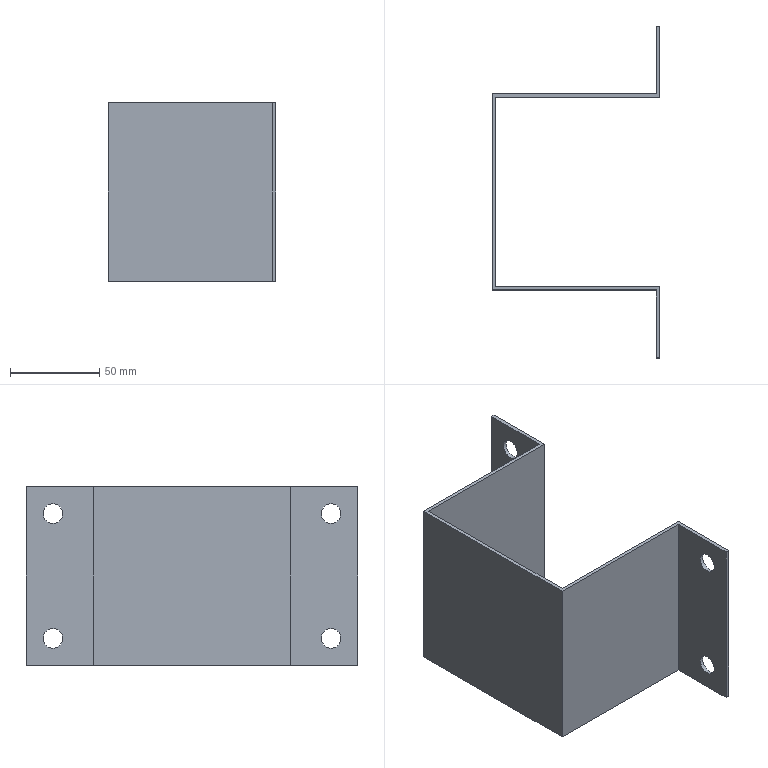Part | NX | features solid 2 | 1 solid | 18 faces | box 94 x 186 x 100 mm | volume 73240 mm3 | plane 14 | cylinder 4 | commonest cylinder face diameters 11 x4
STEP:
#1=CARTESIAN_POINT('',(1132.,-77.,-389.5));
#2=VERTEX_POINT('',#1);
#3=CARTESIAN_POINT('',(1132.,-77.,-395.));
#4=DIRECTION('',(-1.,0.,0.));
#5=DIRECTION('',(0.,0.,1.));
#6=AXIS2_PLACEMENT_3D('',#3,#4,#5);
#7=CIRCLE('',#6,5.5);
#8=EDGE_CURVE('',#2,#2,#7,.F.);
#9=ORIENTED_EDGE('',*,*,#8,.F.);
#10=EDGE_LOOP('',(#9));
#11=FACE_BOUND('',#10,.T.);
#12=CARTESIAN_POINT('',(1132.,-102.,-480.));
#13=VERTEX_POINT('',#12);
#14=CARTESIAN_POINT('',(1132.,-62.,-480.));
#15=VERTEX_POINT('',#14);
#16=CARTESIAN_POINT('',(1132.,-74.,-480.));
#17=DIRECTION('',(0.,1.,0.));
#18=VECTOR('',#17,1000.);
#19=LINE('',#16,#18);
#20=EDGE_CURVE('',#13,#15,#19,.T.);
#21=ORIENTED_EDGE('',*,*,#20,.T.);
#22=CARTESIAN_POINT('',(1132.,-62.,-380.));
#23=VERTEX_POINT('',#22);
#24=CARTESIAN_POINT('',(1132.,-62.,-480.));
#25=DIRECTION('',(0.,0.,1.));
#26=VECTOR('',#25,1000.);
#27=LINE('',#24,#26);
#28=EDGE_CURVE('',#15,#23,#27,.T.);
#29=ORIENTED_EDGE('',*,*,#28,.T.);
#30=CARTESIAN_POINT('',(1132.,-102.,-380.));
#31=VERTEX_POINT('',#30);
#32=CARTESIAN_POINT('',(1132.,-74.,-380.));
#33=DIRECTION('',(0.,1.,0.));
#34=VECTOR('',#33,1000.);
#35=LINE('',#32,#34);
#36=EDGE_CURVE('',#31,#23,#35,.T.);
#37=ORIENTED_EDGE('',*,*,#36,.F.);
#38=CARTESIAN_POINT('',(1132.,-102.,-480.));
#39=DIRECTION('',(0.,0.,1.));
#40=VECTOR('',#39,1000.);
#41=LINE('',#38,#40);
#42=EDGE_CURVE('',#13,#31,#41,.T.);
#43=ORIENTED_EDGE('',*,*,#42,.F.);
#44=EDGE_LOOP('',(#21,#29,#37,#43));
#45=FACE_BOUND('',#44,.T.);
#46=CARTESIAN_POINT('',(1132.,-77.,-459.5));
#47=VERTEX_POINT('',#46);
#48=CARTESIAN_POINT('',(1132.,-77.,-465.));
#49=DIRECTION('',(-1.,0.,0.));
#50=DIRECTION('',(0.,0.,1.));
#51=AXIS2_PLACEMENT_3D('',#48,#49,#50);
#52=CIRCLE('',#51,5.5);
#53=EDGE_CURVE('',#47,#47,#52,.F.);
#54=ORIENTED_EDGE('',*,*,#53,.F.);
#55=EDGE_LOOP('',(#54));
#56=FACE_BOUND('',#55,.T.);
#57=CARTESIAN_POINT('',(1132.,-74.,-480.));
#58=DIRECTION('',(-1.,0.,0.));
#59=DIRECTION('',(0.,1.,0.));
#60=AXIS2_PLACEMENT_3D('',#57,#58,#59);
#61=PLANE('',#60);
#62=ADVANCED_FACE('',(#11,#45,#56),#61,.F.);
#63=CARTESIAN_POINT('',(1130.,-77.,-389.5));
#64=VERTEX_POINT('',#63);
#65=CARTESIAN_POINT('',(1130.,-77.,-395.));
#66=DIRECTION('',(-1.,0.,0.));
#67=DIRECTION('',(0.,0.,1.));
#68=AXIS2_PLACEMENT_3D('',#65,#66,#67);
#69=CIRCLE('',#68,5.5);
#70=EDGE_CURVE('',#64,#64,#69,.F.);
#71=ORIENTED_EDGE('',*,*,#70,.T.);
#72=EDGE_LOOP('',(#71));
#73=FACE_BOUND('',#72,.T.);
#74=CARTESIAN_POINT('',(1130.,-100.,-480.));
#75=VERTEX_POINT('',#74);
#76=CARTESIAN_POINT('',(1130.,-62.,-480.));
#77=VERTEX_POINT('',#76);
#78=CARTESIAN_POINT('',(1130.,-72.,-480.));
#79=DIRECTION('',(0.,1.,0.));
#80=VECTOR('',#79,1000.);
#81=LINE('',#78,#80);
#82=EDGE_CURVE('',#75,#77,#81,.T.);
#83=ORIENTED_EDGE('',*,*,#82,.F.);
#84=CARTESIAN_POINT('',(1130.,-100.,-380.));
#85=VERTEX_POINT('',#84);
#86=CARTESIAN_POINT('',(1130.,-100.,-480.));
#87=DIRECTION('',(0.,0.,1.));
#88=VECTOR('',#87,1000.);
#89=LINE('',#86,#88);
#90=EDGE_CURVE('',#75,#85,#89,.T.);
#91=ORIENTED_EDGE('',*,*,#90,.T.);
#92=CARTESIAN_POINT('',(1130.,-62.,-380.));
#93=VERTEX_POINT('',#92);
#94=CARTESIAN_POINT('',(1130.,-72.,-380.));
#95=DIRECTION('',(0.,1.,0.));
#96=VECTOR('',#95,1000.);
#97=LINE('',#94,#96);
#98=EDGE_CURVE('',#85,#93,#97,.T.);
#99=ORIENTED_EDGE('',*,*,#98,.T.);
#100=CARTESIAN_POINT('',(1130.,-62.,-480.));
#101=DIRECTION('',(0.,0.,1.));
#102=VECTOR('',#101,1000.);
#103=LINE('',#100,#102);
#104=EDGE_CURVE('',#77,#93,#103,.T.);
#105=ORIENTED_EDGE('',*,*,#104,.F.);
#106=EDGE_LOOP('',(#83,#91,#99,#105));
#107=FACE_BOUND('',#106,.T.);
#108=CARTESIAN_POINT('',(1130.,-77.,-459.5));
#109=VERTEX_POINT('',#108);
#110=CARTESIAN_POINT('',(1130.,-77.,-465.));
#111=DIRECTION('',(-1.,0.,0.));
#112=DIRECTION('',(0.,0.,1.));
#113=AXIS2_PLACEMENT_3D('',#110,#111,#112);
#114=CIRCLE('',#113,5.5);
#115=EDGE_CURVE('',#109,#109,#114,.F.);
#116=ORIENTED_EDGE('',*,*,#115,.T.);
#117=EDGE_LOOP('',(#116));
#118=FACE_BOUND('',#117,.T.);
#119=CARTESIAN_POINT('',(1130.,-72.,-480.));
#120=DIRECTION('',(-1.,0.,0.));
#121=DIRECTION('',(0.,0.,1.));
#122=AXIS2_PLACEMENT_3D('',#119,#120,#121);
#123=PLANE('',#122);
#124=ADVANCED_FACE('',(#73,#107,#118),#123,.T.);
#125=CARTESIAN_POINT('',(1132.,-233.,-389.5));
#126=VERTEX_POINT('',#125);
#127=CARTESIAN_POINT('',(1132.,-233.,-395.));
#128=DIRECTION('',(-1.,0.,0.));
#129=DIRECTION('',(0.,0.,1.));
#130=AXIS2_PLACEMENT_3D('',#127,#128,#129);
#131=CIRCLE('',#130,5.5);
#132=EDGE_CURVE('',#126,#126,#131,.T.);
#133=ORIENTED_EDGE('',*,*,#132,.T.);
#134=EDGE_LOOP('',(#133));
#135=FACE_BOUND('',#134,.T.);
#136=CARTESIAN_POINT('',(1132.,-208.,-380.));
#137=VERTEX_POINT('',#136);
#138=CARTESIAN_POINT('',(1132.,-248.,-380.));
#139=VERTEX_POINT('',#138);
#140=CARTESIAN_POINT('',(1132.,-206.,-380.));
#141=DIRECTION('',(0.,1.,0.));
#142=VECTOR('',#141,1000.);
#143=LINE('',#140,#142);
#144=EDGE_CURVE('',#137,#139,#143,.F.);
#145=ORIENTED_EDGE('',*,*,#144,.T.);
#146=CARTESIAN_POINT('',(1132.,-248.,-480.));
#147=VERTEX_POINT('',#146);
#148=CARTESIAN_POINT('',(1132.,-248.,-480.));
#149=DIRECTION('',(0.,0.,1.));
#150=VECTOR('',#149,1000.);
#151=LINE('',#148,#150);
#152=EDGE_CURVE('',#147,#139,#151,.T.);
#153=ORIENTED_EDGE('',*,*,#152,.F.);
#154=CARTESIAN_POINT('',(1132.,-208.,-480.));
#155=VERTEX_POINT('',#154);
#156=CARTESIAN_POINT('',(1132.,-206.,-480.));
#157=DIRECTION('',(0.,1.,0.));
#158=VECTOR('',#157,1000.);
#159=LINE('',#156,#158);
#160=EDGE_CURVE('',#155,#147,#159,.F.);
#161=ORIENTED_EDGE('',*,*,#160,.F.);
#162=CARTESIAN_POINT('',(1132.,-208.,-480.));
#163=DIRECTION('',(0.,0.,-1.));
#164=VECTOR('',#163,1000.);
#165=LINE('',#162,#164);
#166=EDGE_CURVE('',#155,#137,#165,.F.);
#167=ORIENTED_EDGE('',*,*,#166,.T.);
#168=EDGE_LOOP('',(#145,#153,#161,#167));
#169=FACE_BOUND('',#168,.T.);
#170=CARTESIAN_POINT('',(1132.,-233.,-459.5));
#171=VERTEX_POINT('',#170);
#172=CARTESIAN_POINT('',(1132.,-233.,-465.));
#173=DIRECTION('',(-1.,0.,0.));
#174=DIRECTION('',(0.,0.,1.));
#175=AXIS2_PLACEMENT_3D('',#172,#173,#174);
#176=CIRCLE('',#175,5.5);
#177=EDGE_CURVE('',#171,#171,#176,.T.);
#178=ORIENTED_EDGE('',*,*,#177,.T.);
#179=EDGE_LOOP('',(#178));
#180=FACE_BOUND('',#179,.T.);
#181=CARTESIAN_POINT('',(1132.,-106.,-480.));
#182=DIRECTION('',(-1.,0.,0.));
#183=DIRECTION('',(0.,1.,0.));
#184=AXIS2_PLACEMENT_3D('',#181,#182,#183);
#185=PLANE('',#184);
#186=ADVANCED_FACE('',(#135,#169,#180),#185,.F.);
#187=CARTESIAN_POINT('',(1130.,-233.,-389.5));
#188=VERTEX_POINT('',#187);
#189=CARTESIAN_POINT('',(1130.,-233.,-395.));
#190=DIRECTION('',(-1.,0.,0.));
#191=DIRECTION('',(0.,0.,1.));
#192=AXIS2_PLACEMENT_3D('',#189,#190,#191);
#193=CIRCLE('',#192,5.5);
#194=EDGE_CURVE('',#188,#188,#193,.T.);
#195=ORIENTED_EDGE('',*,*,#194,.F.);
#196=EDGE_LOOP('',(#195));
#197=FACE_BOUND('',#196,.T.);
#198=CARTESIAN_POINT('',(1130.,-210.,-380.));
#199=VERTEX_POINT('',#198);
#200=CARTESIAN_POINT('',(1130.,-248.,-380.));
#201=VERTEX_POINT('',#200);
#202=CARTESIAN_POINT('',(1130.,-208.,-380.));
#203=DIRECTION('',(0.,1.,0.));
#204=VECTOR('',#203,1000.);
#205=LINE('',#202,#204);
#206=EDGE_CURVE('',#199,#201,#205,.F.);
#207=ORIENTED_EDGE('',*,*,#206,.F.);
#208=CARTESIAN_POINT('',(1130.,-210.,-480.));
#209=VERTEX_POINT('',#208);
#210=CARTESIAN_POINT('',(1130.,-210.,-480.));
#211=DIRECTION('',(0.,0.,1.));
#212=VECTOR('',#211,1000.);
#213=LINE('',#210,#212);
#214=EDGE_CURVE('',#199,#209,#213,.F.);
#215=ORIENTED_EDGE('',*,*,#214,.T.);
#216=CARTESIAN_POINT('',(1130.,-248.,-480.));
#217=VERTEX_POINT('',#216);
#218=CARTESIAN_POINT('',(1130.,-208.,-480.));
#219=DIRECTION('',(0.,1.,0.));
#220=VECTOR('',#219,1000.);
#221=LINE('',#218,#220);
#222=EDGE_CURVE('',#209,#217,#221,.F.);
#223=ORIENTED_EDGE('',*,*,#222,.T.);
#224=CARTESIAN_POINT('',(1130.,-248.,-480.));
#225=DIRECTION('',(0.,0.,-1.));
#226=VECTOR('',#225,1000.);
#227=LINE('',#224,#226);
#228=EDGE_CURVE('',#217,#201,#227,.F.);
#229=ORIENTED_EDGE('',*,*,#228,.T.);
#230=EDGE_LOOP('',(#207,#215,#223,#229));
#231=FACE_BOUND('',#230,.T.);
#232=CARTESIAN_POINT('',(1130.,-233.,-459.5));
#233=VERTEX_POINT('',#232);
#234=CARTESIAN_POINT('',(1130.,-233.,-465.));
#235=DIRECTION('',(-1.,0.,0.));
#236=DIRECTION('',(0.,0.,1.));
#237=AXIS2_PLACEMENT_3D('',#234,#235,#236);
#238=CIRCLE('',#237,5.5);
#239=EDGE_CURVE('',#233,#233,#238,.T.);
#240=ORIENTED_EDGE('',*,*,#239,.F.);
#241=EDGE_LOOP('',(#240));
#242=FACE_BOUND('',#241,.T.);
#243=CARTESIAN_POINT('',(1130.,-208.,-480.));
#244=DIRECTION('',(-1.,0.,0.));
#245=DIRECTION('',(0.,0.,1.));
#246=AXIS2_PLACEMENT_3D('',#243,#244,#245);
#247=PLANE('',#246);
#248=ADVANCED_FACE('',(#197,#231,#242),#247,.T.);
#249=CARTESIAN_POINT('',(1038.,-100.,-480.));
#250=VERTEX_POINT('',#249);
#251=CARTESIAN_POINT('',(1040.,-100.,-480.));
#252=DIRECTION('',(1.,0.,0.));
#253=VECTOR('',#252,1000.);
#254=LINE('',#251,#253);
#255=EDGE_CURVE('',#250,#75,#254,.T.);
#256=ORIENTED_EDGE('',*,*,#255,.T.);
#257=ORIENTED_EDGE('',*,*,#82,.T.);
#258=CARTESIAN_POINT('',(1130.,-62.,-480.));
#259=DIRECTION('',(1.,0.,0.));
#260=VECTOR('',#259,1000.);
#261=LINE('',#258,#260);
#262=EDGE_CURVE('',#77,#15,#261,.T.);
#263=ORIENTED_EDGE('',*,*,#262,.T.);
#264=ORIENTED_EDGE('',*,*,#20,.F.);
#265=CARTESIAN_POINT('',(1040.,-102.,-480.));
#266=VERTEX_POINT('',#265);
#267=CARTESIAN_POINT('',(1040.,-102.,-480.));
#268=DIRECTION('',(1.,0.,0.));
#269=VECTOR('',#268,1000.);
#270=LINE('',#267,#269);
#271=EDGE_CURVE('',#266,#13,#270,.T.);
#272=ORIENTED_EDGE('',*,*,#271,.F.);
#273=CARTESIAN_POINT('',(1040.,-208.,-480.));
#274=VERTEX_POINT('',#273);
#275=CARTESIAN_POINT('',(1040.,-206.,-480.));
#276=DIRECTION('',(0.,1.,0.));
#277=VECTOR('',#276,1000.);
#278=LINE('',#275,#277);
#279=EDGE_CURVE('',#274,#266,#278,.T.);
#280=ORIENTED_EDGE('',*,*,#279,.F.);
#281=CARTESIAN_POINT('',(1040.,-208.,-480.));
#282=DIRECTION('',(1.,0.,0.));
#283=VECTOR('',#282,1000.);
#284=LINE('',#281,#283);
#285=EDGE_CURVE('',#274,#155,#284,.T.);
#286=ORIENTED_EDGE('',*,*,#285,.T.);
#287=ORIENTED_EDGE('',*,*,#160,.T.);
#288=CARTESIAN_POINT('',(1130.,-248.,-480.));
#289=DIRECTION('',(1.,0.,0.));
#290=VECTOR('',#289,1000.);
#291=LINE('',#288,#290);
#292=EDGE_CURVE('',#217,#147,#291,.T.);
#293=ORIENTED_EDGE('',*,*,#292,.F.);
#294=ORIENTED_EDGE('',*,*,#222,.F.);
#295=CARTESIAN_POINT('',(1038.,-210.,-480.));
#296=VERTEX_POINT('',#295);
#297=CARTESIAN_POINT('',(1040.,-210.,-480.));
#298=DIRECTION('',(-1.,0.,0.));
#299=VECTOR('',#298,1000.);
#300=LINE('',#297,#299);
#301=EDGE_CURVE('',#296,#209,#300,.F.);
#302=ORIENTED_EDGE('',*,*,#301,.F.);
#303=CARTESIAN_POINT('',(1038.,-206.,-480.));
#304=DIRECTION('',(0.,-1.,0.));
#305=VECTOR('',#304,1000.);
#306=LINE('',#303,#305);
#307=EDGE_CURVE('',#296,#250,#306,.F.);
#308=ORIENTED_EDGE('',*,*,#307,.T.);
#309=EDGE_LOOP('',(#256,#257,#263,#264,#272,#280,#286,#287,#293,#294,#302,#308));
#310=FACE_BOUND('',#309,.T.);
#311=CARTESIAN_POINT('',(1040.,-74.,-480.));
#312=DIRECTION('',(0.,0.,1.));
#313=DIRECTION('',(-1.,0.,0.));
#314=AXIS2_PLACEMENT_3D('',#311,#312,#313);
#315=PLANE('',#314);
#316=ADVANCED_FACE('',(#310),#315,.F.);
#317=CARTESIAN_POINT('',(1040.,-102.,-380.));
#318=VERTEX_POINT('',#317);
#319=CARTESIAN_POINT('',(1040.,-102.,-380.));
#320=DIRECTION('',(1.,0.,0.));
#321=VECTOR('',#320,1000.);
#322=LINE('',#319,#321);
#323=EDGE_CURVE('',#318,#31,#322,.T.);
#324=ORIENTED_EDGE('',*,*,#323,.T.);
#325=ORIENTED_EDGE('',*,*,#36,.T.);
#326=CARTESIAN_POINT('',(1130.,-62.,-380.));
#327=DIRECTION('',(1.,0.,0.));
#328=VECTOR('',#327,1000.);
#329=LINE('',#326,#328);
#330=EDGE_CURVE('',#93,#23,#329,.T.);
#331=ORIENTED_EDGE('',*,*,#330,.F.);
#332=ORIENTED_EDGE('',*,*,#98,.F.);
#333=CARTESIAN_POINT('',(1038.,-100.,-380.));
#334=VERTEX_POINT('',#333);
#335=CARTESIAN_POINT('',(1040.,-100.,-380.));
#336=DIRECTION('',(1.,0.,0.));
#337=VECTOR('',#336,1000.);
#338=LINE('',#335,#337);
#339=EDGE_CURVE('',#334,#85,#338,.T.);
#340=ORIENTED_EDGE('',*,*,#339,.F.);
#341=CARTESIAN_POINT('',(1038.,-210.,-380.));
#342=VERTEX_POINT('',#341);
#343=CARTESIAN_POINT('',(1038.,-206.,-380.));
#344=DIRECTION('',(0.,1.,0.));
#345=VECTOR('',#344,1000.);
#346=LINE('',#343,#345);
#347=EDGE_CURVE('',#342,#334,#346,.T.);
#348=ORIENTED_EDGE('',*,*,#347,.F.);
#349=CARTESIAN_POINT('',(1040.,-210.,-380.));
#350=DIRECTION('',(1.,0.,0.));
#351=VECTOR('',#350,1000.);
#352=LINE('',#349,#351);
#353=EDGE_CURVE('',#342,#199,#352,.T.);
#354=ORIENTED_EDGE('',*,*,#353,.T.);
#355=ORIENTED_EDGE('',*,*,#206,.T.);
#356=CARTESIAN_POINT('',(1130.,-248.,-380.));
#357=DIRECTION('',(-1.,0.,0.));
#358=VECTOR('',#357,1000.);
#359=LINE('',#356,#358);
#360=EDGE_CURVE('',#201,#139,#359,.F.);
#361=ORIENTED_EDGE('',*,*,#360,.T.);
#362=ORIENTED_EDGE('',*,*,#144,.F.);
#363=CARTESIAN_POINT('',(1040.,-208.,-380.));
#364=VERTEX_POINT('',#363);
#365=CARTESIAN_POINT('',(1040.,-208.,-380.));
#366=DIRECTION('',(1.,0.,0.));
#367=VECTOR('',#366,1000.);
#368=LINE('',#365,#367);
#369=EDGE_CURVE('',#364,#137,#368,.T.);
#370=ORIENTED_EDGE('',*,*,#369,.F.);
#371=CARTESIAN_POINT('',(1040.,-206.,-380.));
#372=DIRECTION('',(0.,-1.,0.));
#373=VECTOR('',#372,1000.);
#374=LINE('',#371,#373);
#375=EDGE_CURVE('',#364,#318,#374,.F.);
#376=ORIENTED_EDGE('',*,*,#375,.T.);
#377=EDGE_LOOP('',(#324,#325,#331,#332,#340,#348,#354,#355,#361,#362,#370,#376));
#378=FACE_BOUND('',#377,.T.);
#379=CARTESIAN_POINT('',(1040.,-74.,-380.));
#380=DIRECTION('',(0.,0.,1.));
#381=DIRECTION('',(-1.,0.,0.));
#382=AXIS2_PLACEMENT_3D('',#379,#380,#381);
#383=PLANE('',#382);
#384=ADVANCED_FACE('',(#378),#383,.T.);
#385=ORIENTED_EDGE('',*,*,#271,.T.);
#386=ORIENTED_EDGE('',*,*,#42,.T.);
#387=ORIENTED_EDGE('',*,*,#323,.F.);
#388=CARTESIAN_POINT('',(1040.,-102.,-480.));
#389=DIRECTION('',(0.,0.,1.));
#390=VECTOR('',#389,1000.);
#391=LINE('',#388,#390);
#392=EDGE_CURVE('',#266,#318,#391,.T.);
#393=ORIENTED_EDGE('',*,*,#392,.F.);
#394=EDGE_LOOP('',(#385,#386,#387,#393));
#395=FACE_BOUND('',#394,.T.);
#396=CARTESIAN_POINT('',(1040.,-102.,-480.));
#397=DIRECTION('',(0.,1.,0.));
#398=DIRECTION('',(1.,0.,0.));
#399=AXIS2_PLACEMENT_3D('',#396,#397,#398);
#400=PLANE('',#399);
#401=ADVANCED_FACE('',(#395),#400,.F.);
#402=ORIENTED_EDGE('',*,*,#90,.F.);
#403=ORIENTED_EDGE('',*,*,#255,.F.);
#404=CARTESIAN_POINT('',(1038.,-100.,-480.));
#405=DIRECTION('',(0.,0.,1.));
#406=VECTOR('',#405,1000.);
#407=LINE('',#404,#406);
#408=EDGE_CURVE('',#250,#334,#407,.T.);
#409=ORIENTED_EDGE('',*,*,#408,.T.);
#410=ORIENTED_EDGE('',*,*,#339,.T.);
#411=EDGE_LOOP('',(#402,#403,#409,#410));
#412=FACE_BOUND('',#411,.T.);
#413=CARTESIAN_POINT('',(1040.,-100.,-480.));
#414=DIRECTION('',(0.,1.,0.));
#415=DIRECTION('',(1.,0.,0.));
#416=AXIS2_PLACEMENT_3D('',#413,#414,#415);
#417=PLANE('',#416);
#418=ADVANCED_FACE('',(#412),#417,.T.);
#419=ORIENTED_EDGE('',*,*,#28,.F.);
#420=ORIENTED_EDGE('',*,*,#262,.F.);
#421=ORIENTED_EDGE('',*,*,#104,.T.);
#422=ORIENTED_EDGE('',*,*,#330,.T.);
#423=EDGE_LOOP('',(#419,#420,#421,#422));
#424=FACE_BOUND('',#423,.T.);
#425=CARTESIAN_POINT('',(1130.,-62.,-480.));
#426=DIRECTION('',(0.,1.,0.));
#427=DIRECTION('',(1.,0.,0.));
#428=AXIS2_PLACEMENT_3D('',#425,#426,#427);
#429=PLANE('',#428);
#430=ADVANCED_FACE('',(#424),#429,.T.);
#431=ORIENTED_EDGE('',*,*,#392,.T.);
#432=ORIENTED_EDGE('',*,*,#375,.F.);
#433=CARTESIAN_POINT('',(1040.,-208.,-480.));
#434=DIRECTION('',(0.,0.,-1.));
#435=VECTOR('',#434,1000.);
#436=LINE('',#433,#435);
#437=EDGE_CURVE('',#274,#364,#436,.F.);
#438=ORIENTED_EDGE('',*,*,#437,.F.);
#439=ORIENTED_EDGE('',*,*,#279,.T.);
#440=EDGE_LOOP('',(#431,#432,#438,#439));
#441=FACE_BOUND('',#440,.T.);
#442=CARTESIAN_POINT('',(1040.,-206.,-480.));
#443=DIRECTION('',(-1.,0.,0.));
#444=DIRECTION('',(0.,0.,1.));
#445=AXIS2_PLACEMENT_3D('',#442,#443,#444);
#446=PLANE('',#445);
#447=ADVANCED_FACE('',(#441),#446,.F.);
#448=ORIENTED_EDGE('',*,*,#214,.F.);
#449=ORIENTED_EDGE('',*,*,#353,.F.);
#450=CARTESIAN_POINT('',(1038.,-210.,-480.));
#451=DIRECTION('',(0.,0.,1.));
#452=VECTOR('',#451,1000.);
#453=LINE('',#450,#452);
#454=EDGE_CURVE('',#296,#342,#453,.T.);
#455=ORIENTED_EDGE('',*,*,#454,.F.);
#456=ORIENTED_EDGE('',*,*,#301,.T.);
#457=EDGE_LOOP('',(#448,#449,#455,#456));
#458=FACE_BOUND('',#457,.T.);
#459=CARTESIAN_POINT('',(1040.,-210.,-480.));
#460=DIRECTION('',(0.,1.,0.));
#461=DIRECTION('',(1.,0.,0.));
#462=AXIS2_PLACEMENT_3D('',#459,#460,#461);
#463=PLANE('',#462);
#464=ADVANCED_FACE('',(#458),#463,.F.);
#465=ORIENTED_EDGE('',*,*,#408,.F.);
#466=ORIENTED_EDGE('',*,*,#307,.F.);
#467=ORIENTED_EDGE('',*,*,#454,.T.);
#468=ORIENTED_EDGE('',*,*,#347,.T.);
#469=EDGE_LOOP('',(#465,#466,#467,#468));
#470=FACE_BOUND('',#469,.T.);
#471=CARTESIAN_POINT('',(1038.,-206.,-480.));
#472=DIRECTION('',(-1.,0.,0.));
#473=DIRECTION('',(0.,0.,1.));
#474=AXIS2_PLACEMENT_3D('',#471,#472,#473);
#475=PLANE('',#474);
#476=ADVANCED_FACE('',(#470),#475,.T.);
#477=ORIENTED_EDGE('',*,*,#166,.F.);
#478=ORIENTED_EDGE('',*,*,#285,.F.);
#479=ORIENTED_EDGE('',*,*,#437,.T.);
#480=ORIENTED_EDGE('',*,*,#369,.T.);
#481=EDGE_LOOP('',(#477,#478,#479,#480));
#482=FACE_BOUND('',#481,.T.);
#483=CARTESIAN_POINT('',(1040.,-208.,-480.));
#484=DIRECTION('',(0.,1.,0.));
#485=DIRECTION('',(1.,0.,0.));
#486=AXIS2_PLACEMENT_3D('',#483,#484,#485);
#487=PLANE('',#486);
#488=ADVANCED_FACE('',(#482),#487,.T.);
#489=ORIENTED_EDGE('',*,*,#152,.T.);
#490=ORIENTED_EDGE('',*,*,#360,.F.);
#491=ORIENTED_EDGE('',*,*,#228,.F.);
#492=ORIENTED_EDGE('',*,*,#292,.T.);
#493=EDGE_LOOP('',(#489,#490,#491,#492));
#494=FACE_BOUND('',#493,.T.);
#495=CARTESIAN_POINT('',(1130.,-248.,-480.));
#496=DIRECTION('',(0.,1.,0.));
#497=DIRECTION('',(1.,0.,0.));
#498=AXIS2_PLACEMENT_3D('',#495,#496,#497);
#499=PLANE('',#498);
#500=ADVANCED_FACE('',(#494),#499,.F.);
#501=ORIENTED_EDGE('',*,*,#132,.F.);
#502=EDGE_LOOP('',(#501));
#503=FACE_BOUND('',#502,.T.);
#504=ORIENTED_EDGE('',*,*,#194,.T.);
#505=EDGE_LOOP('',(#504));
#506=FACE_BOUND('',#505,.T.);
#507=CARTESIAN_POINT('',(1112.,-233.,-395.));
#508=DIRECTION('',(1.,0.,0.));
#509=DIRECTION('',(0.,0.,-1.));
#510=AXIS2_PLACEMENT_3D('',#507,#508,#509);
#511=CYLINDRICAL_SURFACE('',#510,5.5);
#512=ADVANCED_FACE('',(#503,#506),#511,.F.);
#513=ORIENTED_EDGE('',*,*,#177,.F.);
#514=EDGE_LOOP('',(#513));
#515=FACE_BOUND('',#514,.T.);
#516=ORIENTED_EDGE('',*,*,#239,.T.);
#517=EDGE_LOOP('',(#516));
#518=FACE_BOUND('',#517,.T.);
#519=CARTESIAN_POINT('',(1112.,-233.,-465.));
#520=DIRECTION('',(1.,0.,0.));
#521=DIRECTION('',(0.,0.,-1.));
#522=AXIS2_PLACEMENT_3D('',#519,#520,#521);
#523=CYLINDRICAL_SURFACE('',#522,5.5);
#524=ADVANCED_FACE('',(#515,#518),#523,.F.);
#525=ORIENTED_EDGE('',*,*,#70,.F.);
#526=EDGE_LOOP('',(#525));
#527=FACE_BOUND('',#526,.T.);
#528=ORIENTED_EDGE('',*,*,#8,.T.);
#529=EDGE_LOOP('',(#528));
#530=FACE_BOUND('',#529,.T.);
#531=CARTESIAN_POINT('',(1112.,-77.,-395.));
#532=DIRECTION('',(1.,0.,0.));
#533=DIRECTION('',(0.,0.,-1.));
#534=AXIS2_PLACEMENT_3D('',#531,#532,#533);
#535=CYLINDRICAL_SURFACE('',#534,5.5);
#536=ADVANCED_FACE('',(#527,#530),#535,.F.);
#537=ORIENTED_EDGE('',*,*,#115,.F.);
#538=EDGE_LOOP('',(#537));
#539=FACE_BOUND('',#538,.T.);
#540=ORIENTED_EDGE('',*,*,#53,.T.);
#541=EDGE_LOOP('',(#540));
#542=FACE_BOUND('',#541,.T.);
#543=CARTESIAN_POINT('',(1112.,-77.,-465.));
#544=DIRECTION('',(1.,0.,0.));
#545=DIRECTION('',(0.,0.,-1.));
#546=AXIS2_PLACEMENT_3D('',#543,#544,#545);
#547=CYLINDRICAL_SURFACE('',#546,5.5);
#548=ADVANCED_FACE('',(#539,#542),#547,.F.);
#549=CLOSED_SHELL('',(#62,#124,#186,#248,#316,#384,#401,#418,#430,#447,#464,#476,#488,#500,#512,#524,#536,#548));
#550=MANIFOLD_SOLID_BREP('',#549);
#551=(LENGTH_UNIT()NAMED_UNIT(*)SI_UNIT(.MILLI.,.METRE.));
#552=UNCERTAINTY_MEASURE_WITH_UNIT(LENGTH_MEASURE(0.00001),#551,'','');
#553=(NAMED_UNIT(*)PLANE_ANGLE_UNIT()SI_UNIT($,.RADIAN.));
#554=(NAMED_UNIT(*)SI_UNIT($,.STERADIAN.)SOLID_ANGLE_UNIT());
#555=(GEOMETRIC_REPRESENTATION_CONTEXT(3)GLOBAL_UNCERTAINTY_ASSIGNED_CONTEXT((#552))GLOBAL_UNIT_ASSIGNED_CONTEXT((#551,#553,#554))REPRESENTATION_CONTEXT('',''));
#556=ADVANCED_BREP_SHAPE_REPRESENTATION('',(#550),#555);